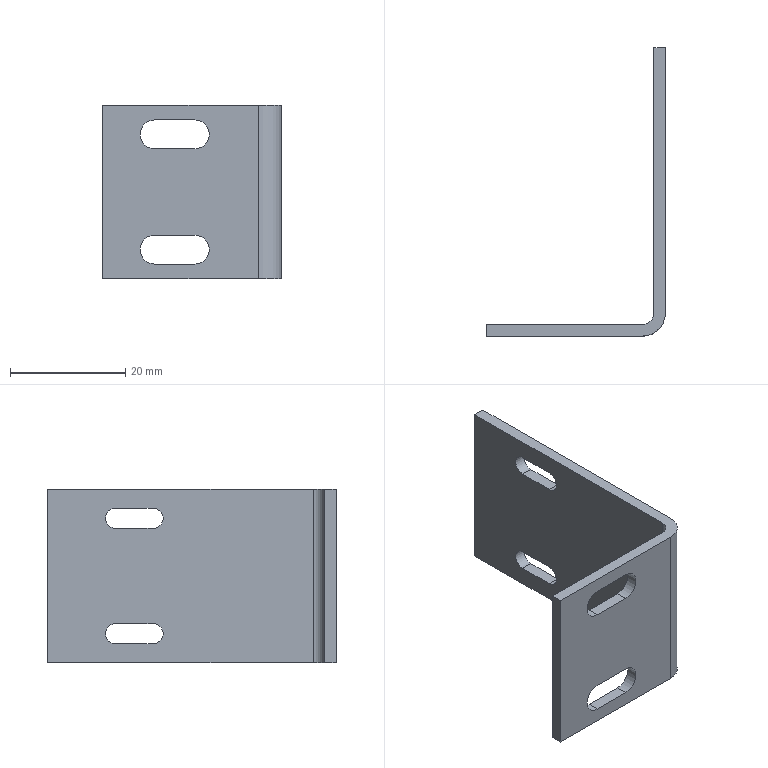Part | STEP file | 0243_208_Plate | 1 solid | 26 faces | box 31 x 50 x 30 mm | volume 4315 mm3 | plane 16 | cylinder 10 | commonest cylinder face diameters 3.5 x4 5 x4 4 x1 8 x1